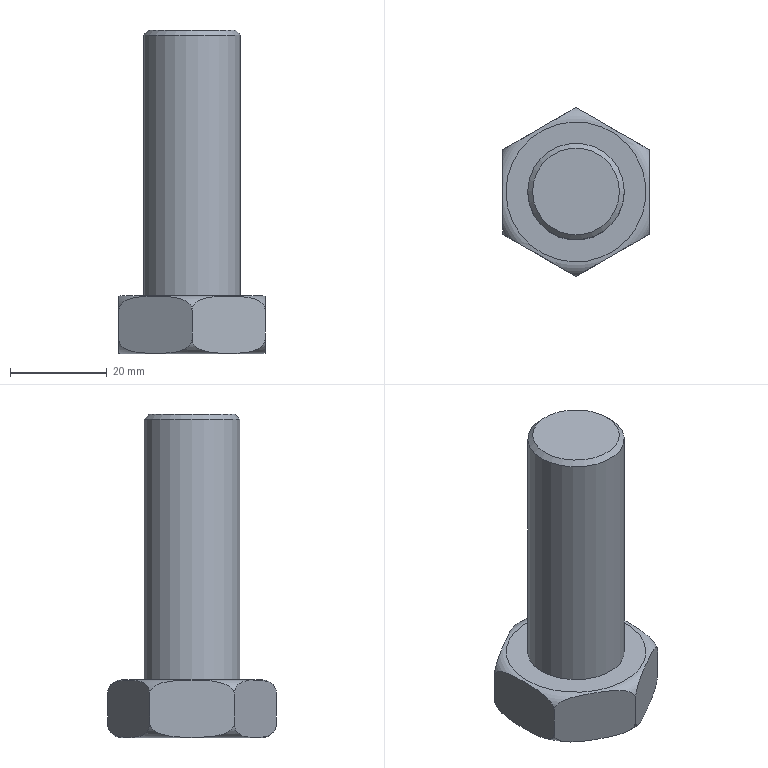Part | NX | features 压板螺钉 2 | 1 solid | 13 faces | box 30.311 x 35 x 67 mm | volume 26733 mm3 | plane 9 | torus 2 | cylinder 1 | cone 1 | commonest cylinder face diameters 20 x1
STEP:
#1=CARTESIAN_POINT('',(-14.5,0.,0.));
#2=VERTEX_POINT('',#1);
#3=CARTESIAN_POINT('',(0.,0.,0.));
#4=DIRECTION('',(0.,0.,-1.));
#5=DIRECTION('',(-1.,0.,0.));
#6=AXIS2_PLACEMENT_3D('',#3,#4,#5);
#7=CIRCLE('',#6,14.5);
#8=EDGE_CURVE('',#2,#2,#7,.F.);
#9=ORIENTED_EDGE('',*,*,#8,.F.);
#10=EDGE_LOOP('',(#9));
#11=FACE_BOUND('',#10,.T.);
#12=CARTESIAN_POINT('',(-15.155,-8.75,-3.));
#13=VERTEX_POINT('',#12);
#14=CARTESIAN_POINT('',(0.,-17.5,-3.));
#15=VERTEX_POINT('',#14);
#16=CARTESIAN_POINT('',(-15.155,-8.75,-3.));
#17=CARTESIAN_POINT('',(-15.155,-8.75,-2.576));
#18=CARTESIAN_POINT('',(-14.824,-8.941,-1.779));
#19=CARTESIAN_POINT('',(-13.614,-9.64,-0.8129));
#20=CARTESIAN_POINT('',(-11.853,-10.657,-0.2974));
#21=CARTESIAN_POINT('',(-9.723,-11.886,-0.09768));
#22=CARTESIAN_POINT('',(-7.57,-13.13,-0.0599));
#23=CARTESIAN_POINT('',(-5.425,-14.368,-0.09759));
#24=CARTESIAN_POINT('',(-3.276,-15.608,-0.3018));
#25=CARTESIAN_POINT('',(-1.53,-16.617,-0.8187));
#26=CARTESIAN_POINT('',(-0.3256,-17.312,-1.787));
#27=CARTESIAN_POINT('',(0.,-17.5,-2.579));
#28=CARTESIAN_POINT('',(0.,-17.5,-3.));
#29=B_SPLINE_CURVE_WITH_KNOTS('',3,(#16,#17,#18,#19,#20,#21,#22,#23,#24,#25,#26,#27,#28),.UNSPECIFIED.,.F.,.F.,(4,1,1,1,1,1,1,1,1,1,4),(0.000000197,0.001252,0.002504,0.005007,0.007511,0.01001,0.01252,0.01502,0.01753,0.01878,0.02003),.UNSPECIFIED.);
#30=EDGE_CURVE('',#13,#15,#29,.T.);
#31=ORIENTED_EDGE('',*,*,#30,.T.);
#32=CARTESIAN_POINT('',(15.155,-8.75,-3.));
#33=VERTEX_POINT('',#32);
#34=CARTESIAN_POINT('',(0.,-17.5,-3.));
#35=CARTESIAN_POINT('',(0.,-17.5,-2.576));
#36=CARTESIAN_POINT('',(0.3312,-17.309,-1.779));
#37=CARTESIAN_POINT('',(1.542,-16.61,-0.8129));
#38=CARTESIAN_POINT('',(3.302,-15.593,-0.2974));
#39=CARTESIAN_POINT('',(5.432,-14.364,-0.09768));
#40=CARTESIAN_POINT('',(7.586,-13.12,-0.0599));
#41=CARTESIAN_POINT('',(9.731,-11.882,-0.09759));
#42=CARTESIAN_POINT('',(11.879,-10.642,-0.3018));
#43=CARTESIAN_POINT('',(13.626,-9.633,-0.8187));
#44=CARTESIAN_POINT('',(14.83,-8.938,-1.787));
#45=CARTESIAN_POINT('',(15.155,-8.75,-2.579));
#46=CARTESIAN_POINT('',(15.155,-8.75,-3.));
#47=B_SPLINE_CURVE_WITH_KNOTS('',3,(#34,#35,#36,#37,#38,#39,#40,#41,#42,#43,#44,#45,#46),.UNSPECIFIED.,.F.,.F.,(4,1,1,1,1,1,1,1,1,1,4),(0.000000197,0.001252,0.002504,0.005007,0.007511,0.01001,0.01252,0.01502,0.01753,0.01878,0.02003),.UNSPECIFIED.);
#48=EDGE_CURVE('',#15,#33,#47,.T.);
#49=ORIENTED_EDGE('',*,*,#48,.T.);
#50=CARTESIAN_POINT('',(15.155,8.75,-3.));
#51=VERTEX_POINT('',#50);
#52=CARTESIAN_POINT('',(15.155,-8.75,-3.));
#53=CARTESIAN_POINT('',(15.155,-8.75,-2.581));
#54=CARTESIAN_POINT('',(15.155,-8.37,-1.78));
#55=CARTESIAN_POINT('',(15.155,-6.973,-0.8148));
#56=CARTESIAN_POINT('',(15.155,-4.938,-0.2973));
#57=CARTESIAN_POINT('',(15.155,-2.482,-0.09825));
#58=CARTESIAN_POINT('',(15.155,-0.008362,-0.05959));
#59=CARTESIAN_POINT('',(15.155,2.473,-0.09827));
#60=CARTESIAN_POINT('',(15.155,4.924,-0.294));
#61=CARTESIAN_POINT('',(15.155,6.978,-0.8172));
#62=CARTESIAN_POINT('',(15.155,8.367,-1.777));
#63=CARTESIAN_POINT('',(15.155,8.75,-2.579));
#64=CARTESIAN_POINT('',(15.155,8.75,-3.));
#65=B_SPLINE_CURVE_WITH_KNOTS('',3,(#52,#53,#54,#55,#56,#57,#58,#59,#60,#61,#62,#63,#64),.UNSPECIFIED.,.F.,.F.,(4,1,1,1,1,1,1,1,1,1,4),(0.02958,0.03081,0.03205,0.03452,0.03699,0.03946,0.04193,0.0444,0.04687,0.0481,0.04934),.UNSPECIFIED.);
#66=EDGE_CURVE('',#33,#51,#65,.T.);
#67=ORIENTED_EDGE('',*,*,#66,.T.);
#68=CARTESIAN_POINT('',(0.,17.5,-3.));
#69=VERTEX_POINT('',#68);
#70=CARTESIAN_POINT('',(15.155,8.75,-3.));
#71=CARTESIAN_POINT('',(15.155,8.75,-2.576));
#72=CARTESIAN_POINT('',(14.824,8.941,-1.779));
#73=CARTESIAN_POINT('',(13.614,9.64,-0.8129));
#74=CARTESIAN_POINT('',(11.853,10.657,-0.2974));
#75=CARTESIAN_POINT('',(9.723,11.886,-0.09768));
#76=CARTESIAN_POINT('',(7.57,13.13,-0.0599));
#77=CARTESIAN_POINT('',(5.425,14.368,-0.09759));
#78=CARTESIAN_POINT('',(3.276,15.608,-0.3018));
#79=CARTESIAN_POINT('',(1.53,16.617,-0.8187));
#80=CARTESIAN_POINT('',(0.3256,17.312,-1.787));
#81=CARTESIAN_POINT('',(0.,17.5,-2.579));
#82=CARTESIAN_POINT('',(0.,17.5,-3.));
#83=B_SPLINE_CURVE_WITH_KNOTS('',3,(#70,#71,#72,#73,#74,#75,#76,#77,#78,#79,#80,#81,#82),.UNSPECIFIED.,.F.,.F.,(4,1,1,1,1,1,1,1,1,1,4),(0.000000197,0.001252,0.002504,0.005007,0.007511,0.01001,0.01252,0.01502,0.01753,0.01878,0.02003),.UNSPECIFIED.);
#84=EDGE_CURVE('',#51,#69,#83,.T.);
#85=ORIENTED_EDGE('',*,*,#84,.T.);
#86=CARTESIAN_POINT('',(-15.155,8.75,-3.));
#87=VERTEX_POINT('',#86);
#88=CARTESIAN_POINT('',(0.,17.5,-3.));
#89=CARTESIAN_POINT('',(0.,17.5,-2.576));
#90=CARTESIAN_POINT('',(-0.3312,17.309,-1.779));
#91=CARTESIAN_POINT('',(-1.542,16.61,-0.8129));
#92=CARTESIAN_POINT('',(-3.302,15.593,-0.2974));
#93=CARTESIAN_POINT('',(-5.432,14.364,-0.09768));
#94=CARTESIAN_POINT('',(-7.586,13.12,-0.0599));
#95=CARTESIAN_POINT('',(-9.731,11.882,-0.09759));
#96=CARTESIAN_POINT('',(-11.879,10.642,-0.3018));
#97=CARTESIAN_POINT('',(-13.626,9.633,-0.8187));
#98=CARTESIAN_POINT('',(-14.83,8.938,-1.787));
#99=CARTESIAN_POINT('',(-15.155,8.75,-2.579));
#100=CARTESIAN_POINT('',(-15.155,8.75,-3.));
#101=B_SPLINE_CURVE_WITH_KNOTS('',3,(#88,#89,#90,#91,#92,#93,#94,#95,#96,#97,#98,#99,#100),.UNSPECIFIED.,.F.,.F.,(4,1,1,1,1,1,1,1,1,1,4),(0.000000197,0.001252,0.002504,0.005007,0.007511,0.01001,0.01252,0.01502,0.01753,0.01878,0.02003),.UNSPECIFIED.);
#102=EDGE_CURVE('',#69,#87,#101,.T.);
#103=ORIENTED_EDGE('',*,*,#102,.T.);
#104=CARTESIAN_POINT('',(-15.155,8.75,-3.));
#105=CARTESIAN_POINT('',(-15.155,8.75,-2.581));
#106=CARTESIAN_POINT('',(-15.155,8.37,-1.78));
#107=CARTESIAN_POINT('',(-15.155,6.973,-0.8148));
#108=CARTESIAN_POINT('',(-15.155,4.938,-0.2973));
#109=CARTESIAN_POINT('',(-15.155,2.482,-0.09825));
#110=CARTESIAN_POINT('',(-15.155,0.008362,-0.05959));
#111=CARTESIAN_POINT('',(-15.155,-2.473,-0.09827));
#112=CARTESIAN_POINT('',(-15.155,-4.924,-0.294));
#113=CARTESIAN_POINT('',(-15.155,-6.978,-0.8172));
#114=CARTESIAN_POINT('',(-15.155,-8.367,-1.777));
#115=CARTESIAN_POINT('',(-15.155,-8.75,-2.579));
#116=CARTESIAN_POINT('',(-15.155,-8.75,-3.));
#117=B_SPLINE_CURVE_WITH_KNOTS('',3,(#104,#105,#106,#107,#108,#109,#110,#111,#112,#113,#114,#115,#116),.UNSPECIFIED.,.F.,.F.,(4,1,1,1,1,1,1,1,1,1,4),(0.02958,0.03081,0.03205,0.03452,0.03699,0.03946,0.04193,0.0444,0.04687,0.0481,0.04934),.UNSPECIFIED.);
#118=EDGE_CURVE('',#87,#13,#117,.T.);
#119=ORIENTED_EDGE('',*,*,#118,.T.);
#120=EDGE_LOOP('',(#31,#49,#67,#85,#103,#119));
#121=FACE_BOUND('',#120,.T.);
#122=CARTESIAN_POINT('',(0.,0.,-3.));
#123=DIRECTION('',(0.,0.,-1.));
#124=DIRECTION('',(-1.,0.,0.));
#125=AXIS2_PLACEMENT_3D('',#122,#123,#124);
#126=TOROIDAL_SURFACE('',#125,14.5,3.);
#127=ADVANCED_FACE('',(#11,#121),#126,.T.);
#128=CARTESIAN_POINT('',(10.,0.,54.));
#129=VERTEX_POINT('',#128);
#130=CARTESIAN_POINT('',(0.,0.,54.));
#131=DIRECTION('',(0.,0.,1.));
#132=DIRECTION('',(1.,0.,0.));
#133=AXIS2_PLACEMENT_3D('',#130,#131,#132);
#134=CIRCLE('',#133,10.);
#135=EDGE_CURVE('',#129,#129,#134,.F.);
#136=ORIENTED_EDGE('',*,*,#135,.T.);
#137=EDGE_LOOP('',(#136));
#138=FACE_BOUND('',#137,.T.);
#139=CARTESIAN_POINT('',(-10.,0.,0.));
#140=VERTEX_POINT('',#139);
#141=CARTESIAN_POINT('',(0.,0.,0.));
#142=DIRECTION('',(0.,0.,-1.));
#143=DIRECTION('',(-1.,0.,0.));
#144=AXIS2_PLACEMENT_3D('',#141,#142,#143);
#145=CIRCLE('',#144,10.);
#146=EDGE_CURVE('',#140,#140,#145,.T.);
#147=ORIENTED_EDGE('',*,*,#146,.F.);
#148=EDGE_LOOP('',(#147));
#149=FACE_BOUND('',#148,.T.);
#150=CARTESIAN_POINT('',(0.,0.,55.));
#151=DIRECTION('',(0.,0.,-1.));
#152=DIRECTION('',(-1.,0.,0.));
#153=AXIS2_PLACEMENT_3D('',#150,#151,#152);
#154=CYLINDRICAL_SURFACE('',#153,10.);
#155=ADVANCED_FACE('',(#138,#149),#154,.T.);
#156=CARTESIAN_POINT('',(9.,0.,55.));
#157=VERTEX_POINT('',#156);
#158=CARTESIAN_POINT('',(0.,0.,55.));
#159=DIRECTION('',(0.,0.,1.));
#160=DIRECTION('',(1.,0.,0.));
#161=AXIS2_PLACEMENT_3D('',#158,#159,#160);
#162=CIRCLE('',#161,9.);
#163=EDGE_CURVE('',#157,#157,#162,.T.);
#164=ORIENTED_EDGE('',*,*,#163,.T.);
#165=EDGE_LOOP('',(#164));
#166=FACE_BOUND('',#165,.T.);
#167=CARTESIAN_POINT('',(0.,0.,55.));
#168=DIRECTION('',(0.,0.,1.));
#169=DIRECTION('',(1.,0.,0.));
#170=AXIS2_PLACEMENT_3D('',#167,#168,#169);
#171=PLANE('',#170);
#172=ADVANCED_FACE('',(#166),#171,.T.);
#173=ORIENTED_EDGE('',*,*,#8,.T.);
#174=EDGE_LOOP('',(#173));
#175=FACE_BOUND('',#174,.T.);
#176=ORIENTED_EDGE('',*,*,#146,.T.);
#177=EDGE_LOOP('',(#176));
#178=FACE_BOUND('',#177,.T.);
#179=CARTESIAN_POINT('',(0.,0.,0.));
#180=DIRECTION('',(0.,0.,-1.));
#181=DIRECTION('',(-1.,0.,0.));
#182=AXIS2_PLACEMENT_3D('',#179,#180,#181);
#183=PLANE('',#182);
#184=ADVANCED_FACE('',(#175,#178),#183,.F.);
#185=CARTESIAN_POINT('',(0.,-17.5,-9.));
#186=VERTEX_POINT('',#185);
#187=CARTESIAN_POINT('',(0.,-17.5,8.));
#188=DIRECTION('',(0.,0.,-1.));
#189=VECTOR('',#188,1000.);
#190=LINE('',#187,#189);
#191=EDGE_CURVE('',#15,#186,#190,.T.);
#192=ORIENTED_EDGE('',*,*,#191,.T.);
#193=CARTESIAN_POINT('',(15.155,-8.75,-9.));
#194=VERTEX_POINT('',#193);
#195=CARTESIAN_POINT('',(15.155,-8.75,-9.));
#196=CARTESIAN_POINT('',(15.155,-8.75,-9.424));
#197=CARTESIAN_POINT('',(14.824,-8.941,-10.221));
#198=CARTESIAN_POINT('',(13.614,-9.64,-11.187));
#199=CARTESIAN_POINT('',(11.853,-10.657,-11.703));
#200=CARTESIAN_POINT('',(9.723,-11.886,-11.902));
#201=CARTESIAN_POINT('',(7.57,-13.13,-11.94));
#202=CARTESIAN_POINT('',(5.425,-14.368,-11.902));
#203=CARTESIAN_POINT('',(3.276,-15.608,-11.698));
#204=CARTESIAN_POINT('',(1.53,-16.617,-11.181));
#205=CARTESIAN_POINT('',(0.3256,-17.312,-10.213));
#206=CARTESIAN_POINT('',(0.,-17.5,-9.421));
#207=CARTESIAN_POINT('',(0.,-17.5,-9.));
#208=B_SPLINE_CURVE_WITH_KNOTS('',3,(#195,#196,#197,#198,#199,#200,#201,#202,#203,#204,#205,#206,#207),.UNSPECIFIED.,.F.,.F.,(4,1,1,1,1,1,1,1,1,1,4),(0.000000197,0.001252,0.002504,0.005007,0.007511,0.01001,0.01252,0.01502,0.01753,0.01878,0.02003),.UNSPECIFIED.);
#209=EDGE_CURVE('',#194,#186,#208,.T.);
#210=ORIENTED_EDGE('',*,*,#209,.F.);
#211=CARTESIAN_POINT('',(15.155,-8.75,8.));
#212=DIRECTION('',(0.,0.,-1.));
#213=VECTOR('',#212,1000.);
#214=LINE('',#211,#213);
#215=EDGE_CURVE('',#33,#194,#214,.T.);
#216=ORIENTED_EDGE('',*,*,#215,.F.);
#217=ORIENTED_EDGE('',*,*,#48,.F.);
#218=EDGE_LOOP('',(#192,#210,#216,#217));
#219=FACE_BOUND('',#218,.T.);
#220=CARTESIAN_POINT('',(15.155,-8.75,8.));
#221=DIRECTION('',(0.5,-0.866,0.));
#222=DIRECTION('',(0.866,0.5,0.));
#223=AXIS2_PLACEMENT_3D('',#220,#221,#222);
#224=PLANE('',#223);
#225=ADVANCED_FACE('',(#219),#224,.T.);
#226=ORIENTED_EDGE('',*,*,#215,.T.);
#227=CARTESIAN_POINT('',(15.155,8.75,-9.));
#228=VERTEX_POINT('',#227);
#229=CARTESIAN_POINT('',(15.155,8.75,-9.));
#230=CARTESIAN_POINT('',(15.155,8.75,-9.419));
#231=CARTESIAN_POINT('',(15.155,8.37,-10.22));
#232=CARTESIAN_POINT('',(15.155,6.973,-11.185));
#233=CARTESIAN_POINT('',(15.155,4.938,-11.703));
#234=CARTESIAN_POINT('',(15.155,2.482,-11.902));
#235=CARTESIAN_POINT('',(15.155,0.008362,-11.94));
#236=CARTESIAN_POINT('',(15.155,-2.473,-11.902));
#237=CARTESIAN_POINT('',(15.155,-4.924,-11.706));
#238=CARTESIAN_POINT('',(15.155,-6.978,-11.183));
#239=CARTESIAN_POINT('',(15.155,-8.367,-10.223));
#240=CARTESIAN_POINT('',(15.155,-8.75,-9.421));
#241=CARTESIAN_POINT('',(15.155,-8.75,-9.));
#242=B_SPLINE_CURVE_WITH_KNOTS('',3,(#229,#230,#231,#232,#233,#234,#235,#236,#237,#238,#239,#240,#241),.UNSPECIFIED.,.F.,.F.,(4,1,1,1,1,1,1,1,1,1,4),(0.02958,0.03081,0.03205,0.03452,0.03699,0.03946,0.04193,0.0444,0.04687,0.0481,0.04934),.UNSPECIFIED.);
#243=EDGE_CURVE('',#228,#194,#242,.T.);
#244=ORIENTED_EDGE('',*,*,#243,.F.);
#245=CARTESIAN_POINT('',(15.155,8.75,8.));
#246=DIRECTION('',(0.,0.,-1.));
#247=VECTOR('',#246,1000.);
#248=LINE('',#245,#247);
#249=EDGE_CURVE('',#51,#228,#248,.T.);
#250=ORIENTED_EDGE('',*,*,#249,.F.);
#251=ORIENTED_EDGE('',*,*,#66,.F.);
#252=EDGE_LOOP('',(#226,#244,#250,#251));
#253=FACE_BOUND('',#252,.T.);
#254=CARTESIAN_POINT('',(15.155,8.75,8.));
#255=DIRECTION('',(1.,0.,0.));
#256=DIRECTION('',(0.,1.,0.));
#257=AXIS2_PLACEMENT_3D('',#254,#255,#256);
#258=PLANE('',#257);
#259=ADVANCED_FACE('',(#253),#258,.T.);
#260=ORIENTED_EDGE('',*,*,#249,.T.);
#261=CARTESIAN_POINT('',(0.,17.5,-9.));
#262=VERTEX_POINT('',#261);
#263=CARTESIAN_POINT('',(0.,17.5,-9.));
#264=CARTESIAN_POINT('',(0.,17.5,-9.424));
#265=CARTESIAN_POINT('',(0.3312,17.309,-10.221));
#266=CARTESIAN_POINT('',(1.542,16.61,-11.187));
#267=CARTESIAN_POINT('',(3.302,15.593,-11.703));
#268=CARTESIAN_POINT('',(5.432,14.364,-11.902));
#269=CARTESIAN_POINT('',(7.586,13.12,-11.94));
#270=CARTESIAN_POINT('',(9.731,11.882,-11.902));
#271=CARTESIAN_POINT('',(11.879,10.642,-11.698));
#272=CARTESIAN_POINT('',(13.626,9.633,-11.181));
#273=CARTESIAN_POINT('',(14.83,8.938,-10.213));
#274=CARTESIAN_POINT('',(15.155,8.75,-9.421));
#275=CARTESIAN_POINT('',(15.155,8.75,-9.));
#276=B_SPLINE_CURVE_WITH_KNOTS('',3,(#263,#264,#265,#266,#267,#268,#269,#270,#271,#272,#273,#274,#275),.UNSPECIFIED.,.F.,.F.,(4,1,1,1,1,1,1,1,1,1,4),(0.000000197,0.001252,0.002504,0.005007,0.007511,0.01001,0.01252,0.01502,0.01753,0.01878,0.02003),.UNSPECIFIED.);
#277=EDGE_CURVE('',#262,#228,#276,.T.);
#278=ORIENTED_EDGE('',*,*,#277,.F.);
#279=CARTESIAN_POINT('',(0.,17.5,8.));
#280=DIRECTION('',(0.,0.,-1.));
#281=VECTOR('',#280,1000.);
#282=LINE('',#279,#281);
#283=EDGE_CURVE('',#69,#262,#282,.T.);
#284=ORIENTED_EDGE('',*,*,#283,.F.);
#285=ORIENTED_EDGE('',*,*,#84,.F.);
#286=EDGE_LOOP('',(#260,#278,#284,#285));
#287=FACE_BOUND('',#286,.T.);
#288=CARTESIAN_POINT('',(0.,17.5,8.));
#289=DIRECTION('',(0.5,0.866,0.));
#290=DIRECTION('',(-0.866,0.5,0.));
#291=AXIS2_PLACEMENT_3D('',#288,#289,#290);
#292=PLANE('',#291);
#293=ADVANCED_FACE('',(#287),#292,.T.);
#294=ORIENTED_EDGE('',*,*,#283,.T.);
#295=CARTESIAN_POINT('',(-15.155,8.75,-9.));
#296=VERTEX_POINT('',#295);
#297=CARTESIAN_POINT('',(-15.155,8.75,-9.));
#298=CARTESIAN_POINT('',(-15.155,8.75,-9.424));
#299=CARTESIAN_POINT('',(-14.824,8.941,-10.221));
#300=CARTESIAN_POINT('',(-13.614,9.64,-11.187));
#301=CARTESIAN_POINT('',(-11.853,10.657,-11.703));
#302=CARTESIAN_POINT('',(-9.723,11.886,-11.902));
#303=CARTESIAN_POINT('',(-7.57,13.13,-11.94));
#304=CARTESIAN_POINT('',(-5.425,14.368,-11.902));
#305=CARTESIAN_POINT('',(-3.276,15.608,-11.698));
#306=CARTESIAN_POINT('',(-1.53,16.617,-11.181));
#307=CARTESIAN_POINT('',(-0.3256,17.312,-10.213));
#308=CARTESIAN_POINT('',(0.,17.5,-9.421));
#309=CARTESIAN_POINT('',(0.,17.5,-9.));
#310=B_SPLINE_CURVE_WITH_KNOTS('',3,(#297,#298,#299,#300,#301,#302,#303,#304,#305,#306,#307,#308,#309),.UNSPECIFIED.,.F.,.F.,(4,1,1,1,1,1,1,1,1,1,4),(0.000000197,0.001252,0.002504,0.005007,0.007511,0.01001,0.01252,0.01502,0.01753,0.01878,0.02003),.UNSPECIFIED.);
#311=EDGE_CURVE('',#296,#262,#310,.T.);
#312=ORIENTED_EDGE('',*,*,#311,.F.);
#313=CARTESIAN_POINT('',(-15.155,8.75,8.));
#314=DIRECTION('',(0.,0.,-1.));
#315=VECTOR('',#314,1000.);
#316=LINE('',#313,#315);
#317=EDGE_CURVE('',#87,#296,#316,.T.);
#318=ORIENTED_EDGE('',*,*,#317,.F.);
#319=ORIENTED_EDGE('',*,*,#102,.F.);
#320=EDGE_LOOP('',(#294,#312,#318,#319));
#321=FACE_BOUND('',#320,.T.);
#322=CARTESIAN_POINT('',(-15.155,8.75,8.));
#323=DIRECTION('',(-0.5,0.866,0.));
#324=DIRECTION('',(-0.866,-0.5,0.));
#325=AXIS2_PLACEMENT_3D('',#322,#323,#324);
#326=PLANE('',#325);
#327=ADVANCED_FACE('',(#321),#326,.T.);
#328=ORIENTED_EDGE('',*,*,#317,.T.);
#329=CARTESIAN_POINT('',(-15.155,-8.75,-9.));
#330=VERTEX_POINT('',#329);
#331=CARTESIAN_POINT('',(-15.155,-8.75,-9.));
#332=CARTESIAN_POINT('',(-15.155,-8.75,-9.419));
#333=CARTESIAN_POINT('',(-15.155,-8.37,-10.22));
#334=CARTESIAN_POINT('',(-15.155,-6.973,-11.185));
#335=CARTESIAN_POINT('',(-15.155,-4.938,-11.703));
#336=CARTESIAN_POINT('',(-15.155,-2.482,-11.902));
#337=CARTESIAN_POINT('',(-15.155,-0.008362,-11.94));
#338=CARTESIAN_POINT('',(-15.155,2.473,-11.902));
#339=CARTESIAN_POINT('',(-15.155,4.924,-11.706));
#340=CARTESIAN_POINT('',(-15.155,6.978,-11.183));
#341=CARTESIAN_POINT('',(-15.155,8.367,-10.223));
#342=CARTESIAN_POINT('',(-15.155,8.75,-9.421));
#343=CARTESIAN_POINT('',(-15.155,8.75,-9.));
#344=B_SPLINE_CURVE_WITH_KNOTS('',3,(#331,#332,#333,#334,#335,#336,#337,#338,#339,#340,#341,#342,#343),.UNSPECIFIED.,.F.,.F.,(4,1,1,1,1,1,1,1,1,1,4),(0.02958,0.03081,0.03205,0.03452,0.03699,0.03946,0.04193,0.0444,0.04687,0.0481,0.04934),.UNSPECIFIED.);
#345=EDGE_CURVE('',#330,#296,#344,.T.);
#346=ORIENTED_EDGE('',*,*,#345,.F.);
#347=CARTESIAN_POINT('',(-15.155,-8.75,8.));
#348=DIRECTION('',(0.,0.,-1.));
#349=VECTOR('',#348,1000.);
#350=LINE('',#347,#349);
#351=EDGE_CURVE('',#13,#330,#350,.T.);
#352=ORIENTED_EDGE('',*,*,#351,.F.);
#353=ORIENTED_EDGE('',*,*,#118,.F.);
#354=EDGE_LOOP('',(#328,#346,#352,#353));
#355=FACE_BOUND('',#354,.T.);
#356=CARTESIAN_POINT('',(-15.155,-8.75,8.));
#357=DIRECTION('',(-1.,0.,0.));
#358=DIRECTION('',(0.,-1.,0.));
#359=AXIS2_PLACEMENT_3D('',#356,#357,#358);
#360=PLANE('',#359);
#361=ADVANCED_FACE('',(#355),#360,.T.);
#362=ORIENTED_EDGE('',*,*,#351,.T.);
#363=CARTESIAN_POINT('',(0.,-17.5,-9.));
#364=CARTESIAN_POINT('',(0.,-17.5,-9.424));
#365=CARTESIAN_POINT('',(-0.3312,-17.309,-10.221));
#366=CARTESIAN_POINT('',(-1.542,-16.61,-11.187));
#367=CARTESIAN_POINT('',(-3.302,-15.593,-11.703));
#368=CARTESIAN_POINT('',(-5.432,-14.364,-11.902));
#369=CARTESIAN_POINT('',(-7.586,-13.12,-11.94));
#370=CARTESIAN_POINT('',(-9.731,-11.882,-11.902));
#371=CARTESIAN_POINT('',(-11.879,-10.642,-11.698));
#372=CARTESIAN_POINT('',(-13.626,-9.633,-11.181));
#373=CARTESIAN_POINT('',(-14.83,-8.938,-10.213));
#374=CARTESIAN_POINT('',(-15.155,-8.75,-9.421));
#375=CARTESIAN_POINT('',(-15.155,-8.75,-9.));
#376=B_SPLINE_CURVE_WITH_KNOTS('',3,(#363,#364,#365,#366,#367,#368,#369,#370,#371,#372,#373,#374,#375),.UNSPECIFIED.,.F.,.F.,(4,1,1,1,1,1,1,1,1,1,4),(0.000000197,0.001252,0.002504,0.005007,0.007511,0.01001,0.01252,0.01502,0.01753,0.01878,0.02003),.UNSPECIFIED.);
#377=EDGE_CURVE('',#186,#330,#376,.T.);
#378=ORIENTED_EDGE('',*,*,#377,.F.);
#379=ORIENTED_EDGE('',*,*,#191,.F.);
#380=ORIENTED_EDGE('',*,*,#30,.F.);
#381=EDGE_LOOP('',(#362,#378,#379,#380));
#382=FACE_BOUND('',#381,.T.);
#383=CARTESIAN_POINT('',(0.,-17.5,8.));
#384=DIRECTION('',(-0.5,-0.866,0.));
#385=DIRECTION('',(0.866,-0.5,0.));
#386=AXIS2_PLACEMENT_3D('',#383,#384,#385);
#387=PLANE('',#386);
#388=ADVANCED_FACE('',(#382),#387,.T.);
#389=CARTESIAN_POINT('',(-14.5,0.,-12.));
#390=VERTEX_POINT('',#389);
#391=CARTESIAN_POINT('',(0.,0.,-12.));
#392=DIRECTION('',(0.,0.,-1.));
#393=DIRECTION('',(-1.,0.,0.));
#394=AXIS2_PLACEMENT_3D('',#391,#392,#393);
#395=CIRCLE('',#394,14.5);
#396=EDGE_CURVE('',#390,#390,#395,.T.);
#397=ORIENTED_EDGE('',*,*,#396,.T.);
#398=EDGE_LOOP('',(#397));
#399=FACE_BOUND('',#398,.T.);
#400=CARTESIAN_POINT('',(0.,0.,-12.));
#401=DIRECTION('',(0.,0.,-1.));
#402=DIRECTION('',(-1.,0.,0.));
#403=AXIS2_PLACEMENT_3D('',#400,#401,#402);
#404=PLANE('',#403);
#405=ADVANCED_FACE('',(#399),#404,.T.);
#406=ORIENTED_EDGE('',*,*,#396,.F.);
#407=EDGE_LOOP('',(#406));
#408=FACE_BOUND('',#407,.T.);
#409=ORIENTED_EDGE('',*,*,#243,.T.);
#410=ORIENTED_EDGE('',*,*,#209,.T.);
#411=ORIENTED_EDGE('',*,*,#377,.T.);
#412=ORIENTED_EDGE('',*,*,#345,.T.);
#413=ORIENTED_EDGE('',*,*,#311,.T.);
#414=ORIENTED_EDGE('',*,*,#277,.T.);
#415=EDGE_LOOP('',(#409,#410,#411,#412,#413,#414));
#416=FACE_BOUND('',#415,.T.);
#417=CARTESIAN_POINT('',(0.,0.,-9.));
#418=DIRECTION('',(0.,0.,-1.));
#419=DIRECTION('',(-1.,0.,0.));
#420=AXIS2_PLACEMENT_3D('',#417,#418,#419);
#421=TOROIDAL_SURFACE('',#420,14.5,3.);
#422=ADVANCED_FACE('',(#408,#416),#421,.T.);
#423=ORIENTED_EDGE('',*,*,#135,.F.);
#424=EDGE_LOOP('',(#423));
#425=FACE_BOUND('',#424,.T.);
#426=ORIENTED_EDGE('',*,*,#163,.F.);
#427=EDGE_LOOP('',(#426));
#428=FACE_BOUND('',#427,.T.);
#429=CARTESIAN_POINT('',(0.,0.,55.));
#430=DIRECTION('',(0.,0.,-1.));
#431=DIRECTION('',(-1.,0.,0.));
#432=AXIS2_PLACEMENT_3D('',#429,#430,#431);
#433=CONICAL_SURFACE('',#432,9.,0.7854);
#434=ADVANCED_FACE('',(#425,#428),#433,.T.);
#435=CLOSED_SHELL('',(#127,#155,#172,#184,#225,#259,#293,#327,#361,#388,#405,#422,#434));
#436=MANIFOLD_SOLID_BREP('',#435);
#437=(LENGTH_UNIT()NAMED_UNIT(*)SI_UNIT(.MILLI.,.METRE.));
#438=UNCERTAINTY_MEASURE_WITH_UNIT(LENGTH_MEASURE(0.0508),#437,'','');
#439=(NAMED_UNIT(*)PLANE_ANGLE_UNIT()SI_UNIT($,.RADIAN.));
#440=(NAMED_UNIT(*)SI_UNIT($,.STERADIAN.)SOLID_ANGLE_UNIT());
#441=(GEOMETRIC_REPRESENTATION_CONTEXT(3)GLOBAL_UNCERTAINTY_ASSIGNED_CONTEXT((#438))GLOBAL_UNIT_ASSIGNED_CONTEXT((#437,#439,#440))REPRESENTATION_CONTEXT('',''));
#442=ADVANCED_BREP_SHAPE_REPRESENTATION('',(#436),#441);